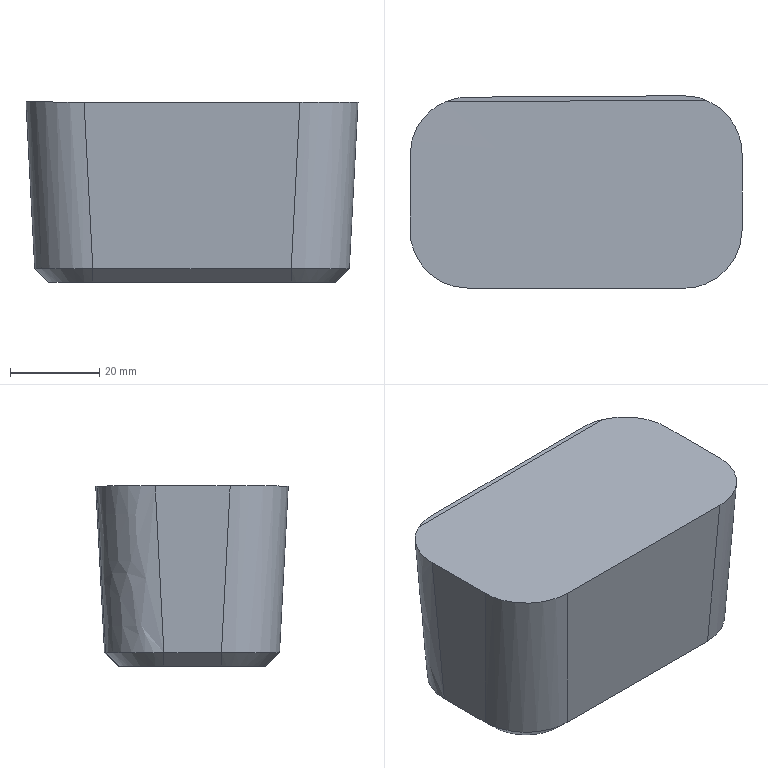Part | STEP file | solid 241 | 1 solid | 24 faces | box 74.217 x 43.029 x 40.25 mm | volume 106174 mm3 | spline 9 | plane 8 | cylinder 4 | cone 2 | other 1 | commonest cylinder face diameters 26 x2 10.2 x1 22 x1